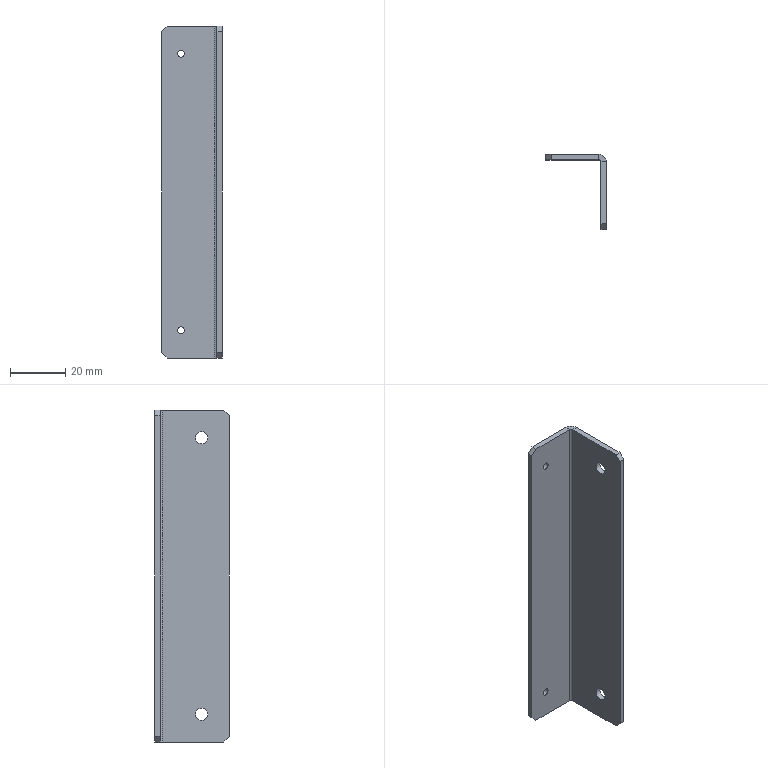Part | NX | 1 solid | 22 faces | box 22 x 27 x 120 mm | volume 11002 mm3 | plane 16 | cylinder 6 | commonest cylinder face diameters 2.5 x2 4.5 x2 1.473 x1 5.473 x1
STEP:
#1=CARTESIAN_POINT('',(-8.,0.,60.));
#2=VERTEX_POINT('',#1);
#3=CARTESIAN_POINT('',(9.263,0.,60.));
#4=VERTEX_POINT('',#3);
#5=CARTESIAN_POINT('',(-10.,0.,60.));
#6=DIRECTION('',(1.,0.,0.));
#7=VECTOR('',#6,1000.);
#8=LINE('',#5,#7);
#9=EDGE_CURVE('',#2,#4,#8,.T.);
#10=ORIENTED_EDGE('',*,*,#9,.F.);
#11=CARTESIAN_POINT('',(-8.,-2.,60.));
#12=VERTEX_POINT('',#11);
#13=CARTESIAN_POINT('',(-8.,-2.,60.));
#14=DIRECTION('',(0.,-1.,0.));
#15=VECTOR('',#14,1000.);
#16=LINE('',#13,#15);
#17=EDGE_CURVE('',#2,#12,#16,.T.);
#18=ORIENTED_EDGE('',*,*,#17,.T.);
#19=CARTESIAN_POINT('',(9.263,-2.,60.));
#20=VERTEX_POINT('',#19);
#21=CARTESIAN_POINT('',(-10.,-2.,60.));
#22=DIRECTION('',(1.,0.,0.));
#23=VECTOR('',#22,1000.);
#24=LINE('',#21,#23);
#25=EDGE_CURVE('',#12,#20,#24,.T.);
#26=ORIENTED_EDGE('',*,*,#25,.T.);
#27=CARTESIAN_POINT('',(9.263,-2.,60.));
#28=DIRECTION('',(0.,1.,0.));
#29=VECTOR('',#28,1000.);
#30=LINE('',#27,#29);
#31=EDGE_CURVE('',#20,#4,#30,.T.);
#32=ORIENTED_EDGE('',*,*,#31,.T.);
#33=EDGE_LOOP('',(#10,#18,#26,#32));
#34=FACE_BOUND('',#33,.T.);
#35=CARTESIAN_POINT('',(-10.,-2.,60.));
#36=DIRECTION('',(0.,0.,1.));
#37=DIRECTION('',(1.,0.,0.));
#38=AXIS2_PLACEMENT_3D('',#35,#36,#37);
#39=PLANE('',#38);
#40=ADVANCED_FACE('',(#34),#39,.T.);
#41=CARTESIAN_POINT('',(-3.,-2.,-51.25));
#42=VERTEX_POINT('',#41);
#43=CARTESIAN_POINT('',(-3.,-2.,-50.));
#44=DIRECTION('',(0.,-1.,0.));
#45=DIRECTION('',(0.,0.,-1.));
#46=AXIS2_PLACEMENT_3D('',#43,#44,#45);
#47=CIRCLE('',#46,1.25);
#48=EDGE_CURVE('',#42,#42,#47,.T.);
#49=ORIENTED_EDGE('',*,*,#48,.F.);
#50=EDGE_LOOP('',(#49));
#51=FACE_BOUND('',#50,.T.);
#52=CARTESIAN_POINT('',(-3.,-2.,48.75));
#53=VERTEX_POINT('',#52);
#54=CARTESIAN_POINT('',(-3.,-2.,50.));
#55=DIRECTION('',(0.,-1.,0.));
#56=DIRECTION('',(0.,0.,-1.));
#57=AXIS2_PLACEMENT_3D('',#54,#55,#56);
#58=CIRCLE('',#57,1.25);
#59=EDGE_CURVE('',#53,#53,#58,.T.);
#60=ORIENTED_EDGE('',*,*,#59,.F.);
#61=EDGE_LOOP('',(#60));
#62=FACE_BOUND('',#61,.T.);
#63=ORIENTED_EDGE('',*,*,#25,.F.);
#64=CARTESIAN_POINT('',(-10.,-2.,58.));
#65=VERTEX_POINT('',#64);
#66=CARTESIAN_POINT('',(-34.,-2.,34.));
#67=DIRECTION('',(0.7071,0.,0.7071));
#68=VECTOR('',#67,1000.);
#69=LINE('',#66,#68);
#70=EDGE_CURVE('',#12,#65,#69,.F.);
#71=ORIENTED_EDGE('',*,*,#70,.T.);
#72=CARTESIAN_POINT('',(-10.,-2.,-58.));
#73=VERTEX_POINT('',#72);
#74=CARTESIAN_POINT('',(-10.,-2.,60.));
#75=DIRECTION('',(0.,0.,1.));
#76=VECTOR('',#75,1000.);
#77=LINE('',#74,#76);
#78=EDGE_CURVE('',#73,#65,#77,.T.);
#79=ORIENTED_EDGE('',*,*,#78,.F.);
#80=CARTESIAN_POINT('',(-8.,-2.,-60.));
#81=VERTEX_POINT('',#80);
#82=CARTESIAN_POINT('',(-34.,-2.,-34.));
#83=DIRECTION('',(-0.7071,0.,0.7071));
#84=VECTOR('',#83,1000.);
#85=LINE('',#82,#84);
#86=EDGE_CURVE('',#73,#81,#85,.F.);
#87=ORIENTED_EDGE('',*,*,#86,.T.);
#88=CARTESIAN_POINT('',(9.263,-2.,-60.));
#89=VERTEX_POINT('',#88);
#90=CARTESIAN_POINT('',(-10.,-2.,-60.));
#91=DIRECTION('',(-1.,0.,0.));
#92=VECTOR('',#91,1000.);
#93=LINE('',#90,#92);
#94=EDGE_CURVE('',#89,#81,#93,.T.);
#95=ORIENTED_EDGE('',*,*,#94,.F.);
#96=CARTESIAN_POINT('',(9.263,-2.,60.));
#97=DIRECTION('',(0.,0.,1.));
#98=VECTOR('',#97,1000.);
#99=LINE('',#96,#98);
#100=EDGE_CURVE('',#20,#89,#99,.F.);
#101=ORIENTED_EDGE('',*,*,#100,.F.);
#102=EDGE_LOOP('',(#63,#71,#79,#87,#95,#101));
#103=FACE_BOUND('',#102,.T.);
#104=CARTESIAN_POINT('',(0.,-2.,0.));
#105=DIRECTION('',(0.,-1.,0.));
#106=DIRECTION('',(0.,0.,-1.));
#107=AXIS2_PLACEMENT_3D('',#104,#105,#106);
#108=PLANE('',#107);
#109=ADVANCED_FACE('',(#51,#62,#103),#108,.T.);
#110=CARTESIAN_POINT('',(-3.,0.,-48.75));
#111=VERTEX_POINT('',#110);
#112=CARTESIAN_POINT('',(-3.,0.,-50.));
#113=DIRECTION('',(0.,1.,0.));
#114=DIRECTION('',(0.,0.,1.));
#115=AXIS2_PLACEMENT_3D('',#112,#113,#114);
#116=CIRCLE('',#115,1.25);
#117=EDGE_CURVE('',#111,#111,#116,.T.);
#118=ORIENTED_EDGE('',*,*,#117,.F.);
#119=EDGE_LOOP('',(#118));
#120=FACE_BOUND('',#119,.T.);
#121=CARTESIAN_POINT('',(-3.,0.,51.25));
#122=VERTEX_POINT('',#121);
#123=CARTESIAN_POINT('',(-3.,0.,50.));
#124=DIRECTION('',(0.,1.,0.));
#125=DIRECTION('',(0.,0.,1.));
#126=AXIS2_PLACEMENT_3D('',#123,#124,#125);
#127=CIRCLE('',#126,1.25);
#128=EDGE_CURVE('',#122,#122,#127,.T.);
#129=ORIENTED_EDGE('',*,*,#128,.F.);
#130=EDGE_LOOP('',(#129));
#131=FACE_BOUND('',#130,.T.);
#132=CARTESIAN_POINT('',(-10.,0.,-58.));
#133=VERTEX_POINT('',#132);
#134=CARTESIAN_POINT('',(-10.,0.,58.));
#135=VERTEX_POINT('',#134);
#136=CARTESIAN_POINT('',(-10.,0.,60.));
#137=DIRECTION('',(0.,0.,1.));
#138=VECTOR('',#137,1000.);
#139=LINE('',#136,#138);
#140=EDGE_CURVE('',#133,#135,#139,.T.);
#141=ORIENTED_EDGE('',*,*,#140,.T.);
#142=CARTESIAN_POINT('',(-10.,0.,58.));
#143=DIRECTION('',(-0.7071,0.,-0.7071));
#144=VECTOR('',#143,1000.);
#145=LINE('',#142,#144);
#146=EDGE_CURVE('',#135,#2,#145,.F.);
#147=ORIENTED_EDGE('',*,*,#146,.T.);
#148=ORIENTED_EDGE('',*,*,#9,.T.);
#149=CARTESIAN_POINT('',(9.263,0.,-60.));
#150=VERTEX_POINT('',#149);
#151=CARTESIAN_POINT('',(9.263,0.,60.));
#152=DIRECTION('',(0.,0.,1.));
#153=VECTOR('',#152,1000.);
#154=LINE('',#151,#153);
#155=EDGE_CURVE('',#4,#150,#154,.F.);
#156=ORIENTED_EDGE('',*,*,#155,.T.);
#157=CARTESIAN_POINT('',(-8.,0.,-60.));
#158=VERTEX_POINT('',#157);
#159=CARTESIAN_POINT('',(-10.,0.,-60.));
#160=DIRECTION('',(-1.,0.,0.));
#161=VECTOR('',#160,1000.);
#162=LINE('',#159,#161);
#163=EDGE_CURVE('',#150,#158,#162,.T.);
#164=ORIENTED_EDGE('',*,*,#163,.T.);
#165=CARTESIAN_POINT('',(-8.,0.,-60.));
#166=DIRECTION('',(0.7071,0.,-0.7071));
#167=VECTOR('',#166,1000.);
#168=LINE('',#165,#167);
#169=EDGE_CURVE('',#158,#133,#168,.F.);
#170=ORIENTED_EDGE('',*,*,#169,.T.);
#171=EDGE_LOOP('',(#141,#147,#148,#156,#164,#170));
#172=FACE_BOUND('',#171,.T.);
#173=CARTESIAN_POINT('',(0.,0.,0.));
#174=DIRECTION('',(0.,-1.,0.));
#175=DIRECTION('',(0.,0.,-1.));
#176=AXIS2_PLACEMENT_3D('',#173,#174,#175);
#177=PLANE('',#176);
#178=ADVANCED_FACE('',(#120,#131,#172),#177,.F.);
#179=ORIENTED_EDGE('',*,*,#78,.T.);
#180=CARTESIAN_POINT('',(-10.,-2.,58.));
#181=DIRECTION('',(0.,1.,0.));
#182=VECTOR('',#181,1000.);
#183=LINE('',#180,#182);
#184=EDGE_CURVE('',#65,#135,#183,.T.);
#185=ORIENTED_EDGE('',*,*,#184,.T.);
#186=ORIENTED_EDGE('',*,*,#140,.F.);
#187=CARTESIAN_POINT('',(-10.,-2.,-58.));
#188=DIRECTION('',(0.,-1.,0.));
#189=VECTOR('',#188,1000.);
#190=LINE('',#187,#189);
#191=EDGE_CURVE('',#133,#73,#190,.T.);
#192=ORIENTED_EDGE('',*,*,#191,.T.);
#193=EDGE_LOOP('',(#179,#185,#186,#192));
#194=FACE_BOUND('',#193,.T.);
#195=CARTESIAN_POINT('',(-10.,-2.,60.));
#196=DIRECTION('',(-1.,0.,0.));
#197=DIRECTION('',(0.,0.,1.));
#198=AXIS2_PLACEMENT_3D('',#195,#196,#197);
#199=PLANE('',#198);
#200=ADVANCED_FACE('',(#194),#199,.T.);
#201=ORIENTED_EDGE('',*,*,#94,.T.);
#202=CARTESIAN_POINT('',(-8.,-2.,-60.));
#203=DIRECTION('',(0.,1.,0.));
#204=VECTOR('',#203,1000.);
#205=LINE('',#202,#204);
#206=EDGE_CURVE('',#81,#158,#205,.T.);
#207=ORIENTED_EDGE('',*,*,#206,.T.);
#208=ORIENTED_EDGE('',*,*,#163,.F.);
#209=CARTESIAN_POINT('',(9.263,-2.,-60.));
#210=DIRECTION('',(0.,1.,0.));
#211=VECTOR('',#210,1000.);
#212=LINE('',#209,#211);
#213=EDGE_CURVE('',#89,#150,#212,.T.);
#214=ORIENTED_EDGE('',*,*,#213,.F.);
#215=EDGE_LOOP('',(#201,#207,#208,#214));
#216=FACE_BOUND('',#215,.T.);
#217=CARTESIAN_POINT('',(-10.,-2.,-60.));
#218=DIRECTION('',(0.,0.,-1.));
#219=DIRECTION('',(-1.,0.,0.));
#220=AXIS2_PLACEMENT_3D('',#217,#218,#219);
#221=PLANE('',#220);
#222=ADVANCED_FACE('',(#216),#221,.T.);
#223=CARTESIAN_POINT('',(10.,-2.737,-60.));
#224=VERTEX_POINT('',#223);
#225=CARTESIAN_POINT('',(12.,-2.737,-60.));
#226=VERTEX_POINT('',#225);
#227=CARTESIAN_POINT('',(10.,-2.737,-60.));
#228=DIRECTION('',(1.,0.,0.));
#229=VECTOR('',#228,1000.);
#230=LINE('',#227,#229);
#231=EDGE_CURVE('',#224,#226,#230,.T.);
#232=ORIENTED_EDGE('',*,*,#231,.F.);
#233=CARTESIAN_POINT('',(9.263,-2.737,-60.));
#234=DIRECTION('',(0.,0.,1.));
#235=DIRECTION('',(1.,0.,0.));
#236=AXIS2_PLACEMENT_3D('',#233,#234,#235);
#237=CIRCLE('',#236,0.7366);
#238=EDGE_CURVE('',#89,#224,#237,.F.);
#239=ORIENTED_EDGE('',*,*,#238,.F.);
#240=ORIENTED_EDGE('',*,*,#213,.T.);
#241=CARTESIAN_POINT('',(9.263,-2.737,-60.));
#242=DIRECTION('',(0.,0.,1.));
#243=DIRECTION('',(1.,0.,0.));
#244=AXIS2_PLACEMENT_3D('',#241,#242,#243);
#245=CIRCLE('',#244,2.737);
#246=EDGE_CURVE('',#150,#226,#245,.F.);
#247=ORIENTED_EDGE('',*,*,#246,.T.);
#248=EDGE_LOOP('',(#232,#239,#240,#247));
#249=FACE_BOUND('',#248,.T.);
#250=CARTESIAN_POINT('',(9.263,-2.737,-60.));
#251=DIRECTION('',(0.,0.,-1.));
#252=DIRECTION('',(-1.,0.,0.));
#253=AXIS2_PLACEMENT_3D('',#250,#251,#252);
#254=PLANE('',#253);
#255=ADVANCED_FACE('',(#249),#254,.T.);
#256=CARTESIAN_POINT('',(10.,-2.737,60.));
#257=VERTEX_POINT('',#256);
#258=CARTESIAN_POINT('',(9.263,-2.737,60.));
#259=DIRECTION('',(0.,0.,1.));
#260=DIRECTION('',(1.,0.,0.));
#261=AXIS2_PLACEMENT_3D('',#258,#259,#260);
#262=CIRCLE('',#261,0.7366);
#263=EDGE_CURVE('',#257,#20,#262,.T.);
#264=ORIENTED_EDGE('',*,*,#263,.F.);
#265=CARTESIAN_POINT('',(12.,-2.737,60.));
#266=VERTEX_POINT('',#265);
#267=CARTESIAN_POINT('',(10.,-2.737,60.));
#268=DIRECTION('',(1.,0.,0.));
#269=VECTOR('',#268,1000.);
#270=LINE('',#267,#269);
#271=EDGE_CURVE('',#257,#266,#270,.T.);
#272=ORIENTED_EDGE('',*,*,#271,.T.);
#273=CARTESIAN_POINT('',(9.263,-2.737,60.));
#274=DIRECTION('',(0.,0.,1.));
#275=DIRECTION('',(1.,0.,0.));
#276=AXIS2_PLACEMENT_3D('',#273,#274,#275);
#277=CIRCLE('',#276,2.737);
#278=EDGE_CURVE('',#266,#4,#277,.T.);
#279=ORIENTED_EDGE('',*,*,#278,.T.);
#280=ORIENTED_EDGE('',*,*,#31,.F.);
#281=EDGE_LOOP('',(#264,#272,#279,#280));
#282=FACE_BOUND('',#281,.T.);
#283=CARTESIAN_POINT('',(9.263,-2.737,60.));
#284=DIRECTION('',(0.,0.,-1.));
#285=DIRECTION('',(-1.,0.,0.));
#286=AXIS2_PLACEMENT_3D('',#283,#284,#285);
#287=PLANE('',#286);
#288=ADVANCED_FACE('',(#282),#287,.F.);
#289=ORIENTED_EDGE('',*,*,#155,.F.);
#290=ORIENTED_EDGE('',*,*,#278,.F.);
#291=CARTESIAN_POINT('',(12.,-2.737,0.));
#292=DIRECTION('',(0.,0.,1.));
#293=VECTOR('',#292,1000.);
#294=LINE('',#291,#293);
#295=EDGE_CURVE('',#226,#266,#294,.T.);
#296=ORIENTED_EDGE('',*,*,#295,.F.);
#297=ORIENTED_EDGE('',*,*,#246,.F.);
#298=EDGE_LOOP('',(#289,#290,#296,#297));
#299=FACE_BOUND('',#298,.T.);
#300=CARTESIAN_POINT('',(9.263,-2.737,60.));
#301=DIRECTION('',(0.,0.,1.));
#302=DIRECTION('',(1.,0.,0.));
#303=AXIS2_PLACEMENT_3D('',#300,#301,#302);
#304=CYLINDRICAL_SURFACE('',#303,2.737);
#305=ADVANCED_FACE('',(#299),#304,.T.);
#306=ORIENTED_EDGE('',*,*,#100,.T.);
#307=ORIENTED_EDGE('',*,*,#238,.T.);
#308=CARTESIAN_POINT('',(10.,-2.737,-60.));
#309=DIRECTION('',(0.,0.,1.));
#310=VECTOR('',#309,1000.);
#311=LINE('',#308,#310);
#312=EDGE_CURVE('',#224,#257,#311,.T.);
#313=ORIENTED_EDGE('',*,*,#312,.T.);
#314=ORIENTED_EDGE('',*,*,#263,.T.);
#315=EDGE_LOOP('',(#306,#307,#313,#314));
#316=FACE_BOUND('',#315,.T.);
#317=CARTESIAN_POINT('',(9.263,-2.737,60.));
#318=DIRECTION('',(0.,0.,1.));
#319=DIRECTION('',(1.,0.,0.));
#320=AXIS2_PLACEMENT_3D('',#317,#318,#319);
#321=CYLINDRICAL_SURFACE('',#320,0.7366);
#322=ADVANCED_FACE('',(#316),#321,.F.);
#323=CARTESIAN_POINT('',(10.,-25.,60.));
#324=VERTEX_POINT('',#323);
#325=CARTESIAN_POINT('',(10.,-2.,60.));
#326=DIRECTION('',(0.,1.,0.));
#327=VECTOR('',#326,1000.);
#328=LINE('',#325,#327);
#329=EDGE_CURVE('',#324,#257,#328,.T.);
#330=ORIENTED_EDGE('',*,*,#329,.F.);
#331=CARTESIAN_POINT('',(12.,-25.,60.));
#332=VERTEX_POINT('',#331);
#333=CARTESIAN_POINT('',(12.,-25.,60.));
#334=DIRECTION('',(1.,0.,0.));
#335=VECTOR('',#334,1000.);
#336=LINE('',#333,#335);
#337=EDGE_CURVE('',#324,#332,#336,.T.);
#338=ORIENTED_EDGE('',*,*,#337,.T.);
#339=CARTESIAN_POINT('',(12.,-2.,60.));
#340=DIRECTION('',(0.,1.,0.));
#341=VECTOR('',#340,1000.);
#342=LINE('',#339,#341);
#343=EDGE_CURVE('',#332,#266,#342,.T.);
#344=ORIENTED_EDGE('',*,*,#343,.T.);
#345=ORIENTED_EDGE('',*,*,#271,.F.);
#346=EDGE_LOOP('',(#330,#338,#344,#345));
#347=FACE_BOUND('',#346,.T.);
#348=CARTESIAN_POINT('',(12.,-2.,60.));
#349=DIRECTION('',(0.,0.,1.));
#350=DIRECTION('',(1.,0.,0.));
#351=AXIS2_PLACEMENT_3D('',#348,#349,#350);
#352=PLANE('',#351);
#353=ADVANCED_FACE('',(#347),#352,.T.);
#354=CARTESIAN_POINT('',(12.,-25.,-60.));
#355=VERTEX_POINT('',#354);
#356=CARTESIAN_POINT('',(12.,-27.,-60.));
#357=DIRECTION('',(0.,-1.,0.));
#358=VECTOR('',#357,1000.);
#359=LINE('',#356,#358);
#360=EDGE_CURVE('',#226,#355,#359,.T.);
#361=ORIENTED_EDGE('',*,*,#360,.T.);
#362=CARTESIAN_POINT('',(10.,-25.,-60.));
#363=VERTEX_POINT('',#362);
#364=CARTESIAN_POINT('',(12.,-25.,-60.));
#365=DIRECTION('',(-1.,0.,0.));
#366=VECTOR('',#365,1000.);
#367=LINE('',#364,#366);
#368=EDGE_CURVE('',#355,#363,#367,.T.);
#369=ORIENTED_EDGE('',*,*,#368,.T.);
#370=CARTESIAN_POINT('',(10.,-27.,-60.));
#371=DIRECTION('',(0.,-1.,0.));
#372=VECTOR('',#371,1000.);
#373=LINE('',#370,#372);
#374=EDGE_CURVE('',#224,#363,#373,.T.);
#375=ORIENTED_EDGE('',*,*,#374,.F.);
#376=ORIENTED_EDGE('',*,*,#231,.T.);
#377=EDGE_LOOP('',(#361,#369,#375,#376));
#378=FACE_BOUND('',#377,.T.);
#379=CARTESIAN_POINT('',(12.,-27.,-60.));
#380=DIRECTION('',(0.,0.,-1.));
#381=DIRECTION('',(-1.,0.,0.));
#382=AXIS2_PLACEMENT_3D('',#379,#380,#381);
#383=PLANE('',#382);
#384=ADVANCED_FACE('',(#378),#383,.T.);
#385=CARTESIAN_POINT('',(12.,-17.,-47.75));
#386=VERTEX_POINT('',#385);
#387=CARTESIAN_POINT('',(12.,-17.,-50.));
#388=DIRECTION('',(-1.,0.,0.));
#389=DIRECTION('',(0.,0.,1.));
#390=AXIS2_PLACEMENT_3D('',#387,#388,#389);
#391=CIRCLE('',#390,2.25);
#392=EDGE_CURVE('',#386,#386,#391,.T.);
#393=ORIENTED_EDGE('',*,*,#392,.T.);
#394=EDGE_LOOP('',(#393));
#395=FACE_BOUND('',#394,.T.);
#396=CARTESIAN_POINT('',(12.,-17.,52.25));
#397=VERTEX_POINT('',#396);
#398=CARTESIAN_POINT('',(12.,-17.,50.));
#399=DIRECTION('',(-1.,0.,0.));
#400=DIRECTION('',(0.,0.,1.));
#401=AXIS2_PLACEMENT_3D('',#398,#399,#400);
#402=CIRCLE('',#401,2.25);
#403=EDGE_CURVE('',#397,#397,#402,.T.);
#404=ORIENTED_EDGE('',*,*,#403,.T.);
#405=EDGE_LOOP('',(#404));
#406=FACE_BOUND('',#405,.T.);
#407=CARTESIAN_POINT('',(12.,-27.,-58.));
#408=VERTEX_POINT('',#407);
#409=CARTESIAN_POINT('',(12.,-27.,58.));
#410=VERTEX_POINT('',#409);
#411=CARTESIAN_POINT('',(12.,-27.,60.));
#412=DIRECTION('',(0.,0.,1.));
#413=VECTOR('',#412,1000.);
#414=LINE('',#411,#413);
#415=EDGE_CURVE('',#408,#410,#414,.T.);
#416=ORIENTED_EDGE('',*,*,#415,.F.);
#417=CARTESIAN_POINT('',(12.,-42.5,-42.5));
#418=DIRECTION('',(0.,-0.7071,0.7071));
#419=VECTOR('',#418,1000.);
#420=LINE('',#417,#419);
#421=EDGE_CURVE('',#408,#355,#420,.F.);
#422=ORIENTED_EDGE('',*,*,#421,.T.);
#423=ORIENTED_EDGE('',*,*,#360,.F.);
#424=ORIENTED_EDGE('',*,*,#295,.T.);
#425=ORIENTED_EDGE('',*,*,#343,.F.);
#426=CARTESIAN_POINT('',(12.,-42.5,42.5));
#427=DIRECTION('',(0.,0.7071,0.7071));
#428=VECTOR('',#427,1000.);
#429=LINE('',#426,#428);
#430=EDGE_CURVE('',#332,#410,#429,.F.);
#431=ORIENTED_EDGE('',*,*,#430,.T.);
#432=EDGE_LOOP('',(#416,#422,#423,#424,#425,#431));
#433=FACE_BOUND('',#432,.T.);
#434=CARTESIAN_POINT('',(12.,0.,0.));
#435=DIRECTION('',(1.,0.,0.));
#436=DIRECTION('',(0.,1.,0.));
#437=AXIS2_PLACEMENT_3D('',#434,#435,#436);
#438=PLANE('',#437);
#439=ADVANCED_FACE('',(#395,#406,#433),#438,.T.);
#440=CARTESIAN_POINT('',(10.,-17.,-47.75));
#441=VERTEX_POINT('',#440);
#442=CARTESIAN_POINT('',(10.,-17.,-50.));
#443=DIRECTION('',(-1.,0.,0.));
#444=DIRECTION('',(0.,0.,1.));
#445=AXIS2_PLACEMENT_3D('',#442,#443,#444);
#446=CIRCLE('',#445,2.25);
#447=EDGE_CURVE('',#441,#441,#446,.T.);
#448=ORIENTED_EDGE('',*,*,#447,.F.);
#449=EDGE_LOOP('',(#448));
#450=FACE_BOUND('',#449,.T.);
#451=CARTESIAN_POINT('',(10.,-17.,52.25));
#452=VERTEX_POINT('',#451);
#453=CARTESIAN_POINT('',(10.,-17.,50.));
#454=DIRECTION('',(-1.,0.,0.));
#455=DIRECTION('',(0.,0.,1.));
#456=AXIS2_PLACEMENT_3D('',#453,#454,#455);
#457=CIRCLE('',#456,2.25);
#458=EDGE_CURVE('',#452,#452,#457,.T.);
#459=ORIENTED_EDGE('',*,*,#458,.F.);
#460=EDGE_LOOP('',(#459));
#461=FACE_BOUND('',#460,.T.);
#462=ORIENTED_EDGE('',*,*,#374,.T.);
#463=CARTESIAN_POINT('',(10.,-27.,-58.));
#464=VERTEX_POINT('',#463);
#465=CARTESIAN_POINT('',(10.,-25.,-60.));
#466=DIRECTION('',(0.,0.7071,-0.7071));
#467=VECTOR('',#466,1000.);
#468=LINE('',#465,#467);
#469=EDGE_CURVE('',#363,#464,#468,.F.);
#470=ORIENTED_EDGE('',*,*,#469,.T.);
#471=CARTESIAN_POINT('',(10.,-27.,58.));
#472=VERTEX_POINT('',#471);
#473=CARTESIAN_POINT('',(10.,-27.,60.));
#474=DIRECTION('',(0.,0.,1.));
#475=VECTOR('',#474,1000.);
#476=LINE('',#473,#475);
#477=EDGE_CURVE('',#464,#472,#476,.T.);
#478=ORIENTED_EDGE('',*,*,#477,.T.);
#479=CARTESIAN_POINT('',(10.,-27.,58.));
#480=DIRECTION('',(0.,-0.7071,-0.7071));
#481=VECTOR('',#480,1000.);
#482=LINE('',#479,#481);
#483=EDGE_CURVE('',#472,#324,#482,.F.);
#484=ORIENTED_EDGE('',*,*,#483,.T.);
#485=ORIENTED_EDGE('',*,*,#329,.T.);
#486=ORIENTED_EDGE('',*,*,#312,.F.);
#487=EDGE_LOOP('',(#462,#470,#478,#484,#485,#486));
#488=FACE_BOUND('',#487,.T.);
#489=CARTESIAN_POINT('',(10.,0.,0.));
#490=DIRECTION('',(1.,0.,0.));
#491=DIRECTION('',(0.,1.,0.));
#492=AXIS2_PLACEMENT_3D('',#489,#490,#491);
#493=PLANE('',#492);
#494=ADVANCED_FACE('',(#450,#461,#488),#493,.F.);
#495=ORIENTED_EDGE('',*,*,#477,.F.);
#496=CARTESIAN_POINT('',(12.,-27.,-58.));
#497=DIRECTION('',(1.,0.,0.));
#498=VECTOR('',#497,1000.);
#499=LINE('',#496,#498);
#500=EDGE_CURVE('',#464,#408,#499,.T.);
#501=ORIENTED_EDGE('',*,*,#500,.T.);
#502=ORIENTED_EDGE('',*,*,#415,.T.);
#503=CARTESIAN_POINT('',(12.,-27.,58.));
#504=DIRECTION('',(-1.,0.,0.));
#505=VECTOR('',#504,1000.);
#506=LINE('',#503,#505);
#507=EDGE_CURVE('',#410,#472,#506,.T.);
#508=ORIENTED_EDGE('',*,*,#507,.T.);
#509=EDGE_LOOP('',(#495,#501,#502,#508));
#510=FACE_BOUND('',#509,.T.);
#511=CARTESIAN_POINT('',(12.,-27.,60.));
#512=DIRECTION('',(0.,-1.,0.));
#513=DIRECTION('',(1.,0.,0.));
#514=AXIS2_PLACEMENT_3D('',#511,#512,#513);
#515=PLANE('',#514);
#516=ADVANCED_FACE('',(#510),#515,.T.);
#517=ORIENTED_EDGE('',*,*,#59,.T.);
#518=EDGE_LOOP('',(#517));
#519=FACE_BOUND('',#518,.T.);
#520=ORIENTED_EDGE('',*,*,#128,.T.);
#521=EDGE_LOOP('',(#520));
#522=FACE_BOUND('',#521,.T.);
#523=CARTESIAN_POINT('',(-3.,0.,50.));
#524=DIRECTION('',(0.,1.,0.));
#525=DIRECTION('',(0.,0.,1.));
#526=AXIS2_PLACEMENT_3D('',#523,#524,#525);
#527=CYLINDRICAL_SURFACE('',#526,1.25);
#528=ADVANCED_FACE('',(#519,#522),#527,.F.);
#529=ORIENTED_EDGE('',*,*,#48,.T.);
#530=EDGE_LOOP('',(#529));
#531=FACE_BOUND('',#530,.T.);
#532=ORIENTED_EDGE('',*,*,#117,.T.);
#533=EDGE_LOOP('',(#532));
#534=FACE_BOUND('',#533,.T.);
#535=CARTESIAN_POINT('',(-3.,0.,-50.));
#536=DIRECTION('',(0.,1.,0.));
#537=DIRECTION('',(0.,0.,1.));
#538=AXIS2_PLACEMENT_3D('',#535,#536,#537);
#539=CYLINDRICAL_SURFACE('',#538,1.25);
#540=ADVANCED_FACE('',(#531,#534),#539,.F.);
#541=ORIENTED_EDGE('',*,*,#403,.F.);
#542=EDGE_LOOP('',(#541));
#543=FACE_BOUND('',#542,.T.);
#544=ORIENTED_EDGE('',*,*,#458,.T.);
#545=EDGE_LOOP('',(#544));
#546=FACE_BOUND('',#545,.T.);
#547=CARTESIAN_POINT('',(10.,-17.,50.));
#548=DIRECTION('',(-1.,0.,0.));
#549=DIRECTION('',(0.,0.,1.));
#550=AXIS2_PLACEMENT_3D('',#547,#548,#549);
#551=CYLINDRICAL_SURFACE('',#550,2.25);
#552=ADVANCED_FACE('',(#543,#546),#551,.F.);
#553=ORIENTED_EDGE('',*,*,#392,.F.);
#554=EDGE_LOOP('',(#553));
#555=FACE_BOUND('',#554,.T.);
#556=ORIENTED_EDGE('',*,*,#447,.T.);
#557=EDGE_LOOP('',(#556));
#558=FACE_BOUND('',#557,.T.);
#559=CARTESIAN_POINT('',(10.,-17.,-50.));
#560=DIRECTION('',(-1.,0.,0.));
#561=DIRECTION('',(0.,0.,1.));
#562=AXIS2_PLACEMENT_3D('',#559,#560,#561);
#563=CYLINDRICAL_SURFACE('',#562,2.25);
#564=ADVANCED_FACE('',(#555,#558),#563,.F.);
#565=ORIENTED_EDGE('',*,*,#421,.F.);
#566=ORIENTED_EDGE('',*,*,#500,.F.);
#567=ORIENTED_EDGE('',*,*,#469,.F.);
#568=ORIENTED_EDGE('',*,*,#368,.F.);
#569=EDGE_LOOP('',(#565,#566,#567,#568));
#570=FACE_BOUND('',#569,.T.);
#571=CARTESIAN_POINT('',(12.,-25.,-60.));
#572=DIRECTION('',(0.,0.7071,0.7071));
#573=DIRECTION('',(-1.,0.,0.));
#574=AXIS2_PLACEMENT_3D('',#571,#572,#573);
#575=PLANE('',#574);
#576=ADVANCED_FACE('',(#570),#575,.F.);
#577=ORIENTED_EDGE('',*,*,#430,.F.);
#578=ORIENTED_EDGE('',*,*,#337,.F.);
#579=ORIENTED_EDGE('',*,*,#483,.F.);
#580=ORIENTED_EDGE('',*,*,#507,.F.);
#581=EDGE_LOOP('',(#577,#578,#579,#580));
#582=FACE_BOUND('',#581,.T.);
#583=CARTESIAN_POINT('',(12.,-27.,58.));
#584=DIRECTION('',(0.,0.7071,-0.7071));
#585=DIRECTION('',(-1.,0.,0.));
#586=AXIS2_PLACEMENT_3D('',#583,#584,#585);
#587=PLANE('',#586);
#588=ADVANCED_FACE('',(#582),#587,.F.);
#589=ORIENTED_EDGE('',*,*,#70,.F.);
#590=ORIENTED_EDGE('',*,*,#17,.F.);
#591=ORIENTED_EDGE('',*,*,#146,.F.);
#592=ORIENTED_EDGE('',*,*,#184,.F.);
#593=EDGE_LOOP('',(#589,#590,#591,#592));
#594=FACE_BOUND('',#593,.T.);
#595=CARTESIAN_POINT('',(-10.,-2.,58.));
#596=DIRECTION('',(0.7071,0.,-0.7071));
#597=DIRECTION('',(0.,1.,0.));
#598=AXIS2_PLACEMENT_3D('',#595,#596,#597);
#599=PLANE('',#598);
#600=ADVANCED_FACE('',(#594),#599,.F.);
#601=ORIENTED_EDGE('',*,*,#86,.F.);
#602=ORIENTED_EDGE('',*,*,#191,.F.);
#603=ORIENTED_EDGE('',*,*,#169,.F.);
#604=ORIENTED_EDGE('',*,*,#206,.F.);
#605=EDGE_LOOP('',(#601,#602,#603,#604));
#606=FACE_BOUND('',#605,.T.);
#607=CARTESIAN_POINT('',(-8.,-2.,-60.));
#608=DIRECTION('',(0.7071,0.,0.7071));
#609=DIRECTION('',(0.,1.,0.));
#610=AXIS2_PLACEMENT_3D('',#607,#608,#609);
#611=PLANE('',#610);
#612=ADVANCED_FACE('',(#606),#611,.F.);
#613=CLOSED_SHELL('',(#40,#109,#178,#200,#222,#255,#288,#305,#322,#353,#384,#439,#494,#516,#528,#540,#552,#564,#576,#588,#600,#612));
#614=MANIFOLD_SOLID_BREP('',#613);
#615=(LENGTH_UNIT()NAMED_UNIT(*)SI_UNIT(.MILLI.,.METRE.));
#616=UNCERTAINTY_MEASURE_WITH_UNIT(LENGTH_MEASURE(0.00001),#615,'','');
#617=(NAMED_UNIT(*)PLANE_ANGLE_UNIT()SI_UNIT($,.RADIAN.));
#618=(NAMED_UNIT(*)SI_UNIT($,.STERADIAN.)SOLID_ANGLE_UNIT());
#619=(GEOMETRIC_REPRESENTATION_CONTEXT(3)GLOBAL_UNCERTAINTY_ASSIGNED_CONTEXT((#616))GLOBAL_UNIT_ASSIGNED_CONTEXT((#615,#617,#618))REPRESENTATION_CONTEXT('',''));
#620=ADVANCED_BREP_SHAPE_REPRESENTATION('',(#614),#619);